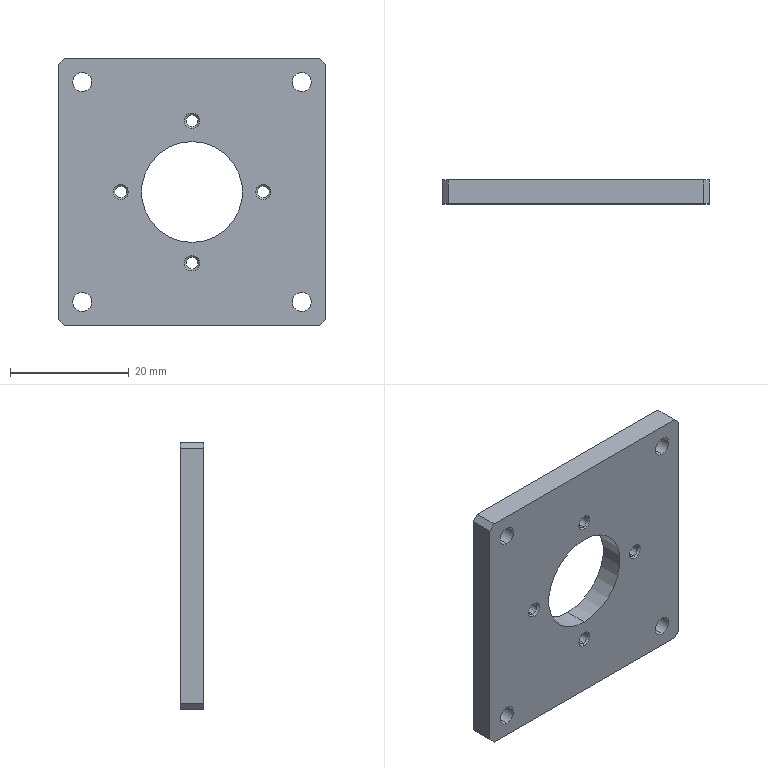Part | SolidWorks | features ICE 5, Chamfer 2, CirPattern 2, Cut 1, Extrusion 1, Fillet 1 | 1 solid | 63 faces | box 45 x 4 x 45 mm | volume 6746 mm3 | cylinder 34 | plane 21 | cone 8 | commonest cylinder face diameters 2 x12 3.2 x8 6 x8 17 x2 22 x2 26 x2